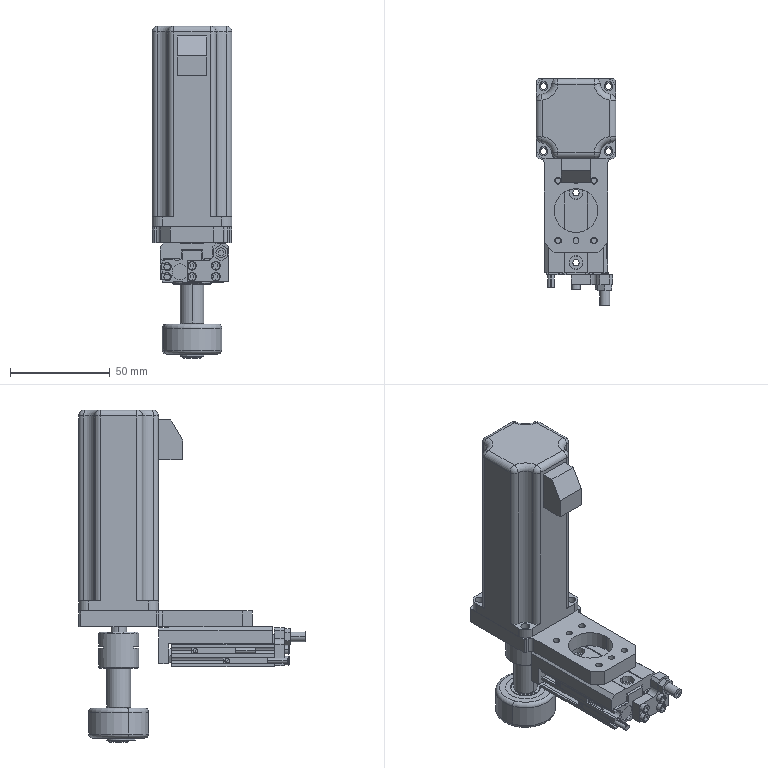Part | SolidWorks | features AEMSimFeature 1 | 13 solids | 652 faces | box 40 x 113.5 x 166.15 mm | volume 207798 mm3 | plane 307 | cylinder 264 | cone 63 | sphere 8 | torus 8 | spline 2 | commonest cylinder face diameters 3 x27 6 x21 4.5 x18 2.013 x16 2.459 x16 10 x14